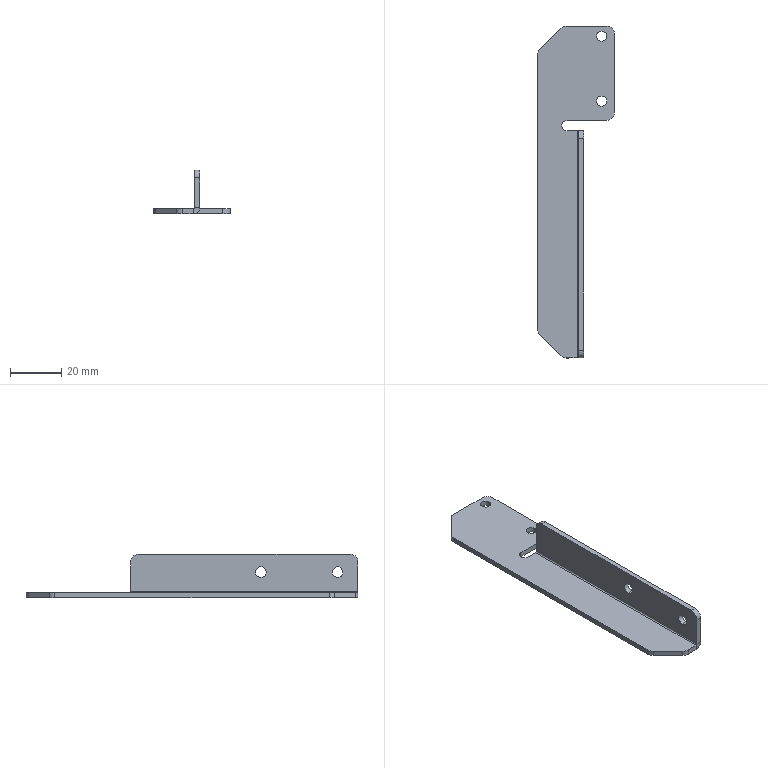Part | SolidWorks | features HoleWzd 2, EdgeFlange 1, Fillet 1, FlatPattern 1, SMBaseFlange 1, SheetMetal 1 | 1 solid | 36 faces | box 30 x 130 x 17 mm | volume 7736 mm3 | cylinder 19 | plane 17 | commonest cylinder face diameters 6 x8 4 x5 4.2 x4 1 x1 5 x1
STEP:
#1=CARTESIAN_POINT('',(23.,116.,-2.));
#2=VERTEX_POINT('',#1);
#3=CARTESIAN_POINT('',(27.,116.,-2.));
#4=VERTEX_POINT('',#3);
#5=CARTESIAN_POINT('',(25.,116.,-2.));
#6=DIRECTION('',(0.,0.,1.));
#7=DIRECTION('',(1.,0.,0.));
#8=AXIS2_PLACEMENT_3D('',#5,#6,#7);
#9=CIRCLE('',#8,2.);
#10=EDGE_CURVE('',#2,#4,#9,.T.);
#11=ORIENTED_EDGE('',*,*,#10,.F.);
#12=CARTESIAN_POINT('',(23.,116.,0.));
#13=VERTEX_POINT('',#12);
#14=CARTESIAN_POINT('',(23.,116.,0.));
#15=DIRECTION('',(0.,0.,1.));
#16=VECTOR('',#15,1000.);
#17=LINE('',#14,#16);
#18=EDGE_CURVE('',#2,#13,#17,.T.);
#19=ORIENTED_EDGE('',*,*,#18,.T.);
#20=CARTESIAN_POINT('',(27.,116.,0.));
#21=VERTEX_POINT('',#20);
#22=CARTESIAN_POINT('',(25.,116.,0.));
#23=DIRECTION('',(0.,0.,1.));
#24=DIRECTION('',(1.,0.,0.));
#25=AXIS2_PLACEMENT_3D('',#22,#23,#24);
#26=CIRCLE('',#25,2.);
#27=EDGE_CURVE('',#13,#21,#26,.T.);
#28=ORIENTED_EDGE('',*,*,#27,.T.);
#29=CARTESIAN_POINT('',(27.,116.,0.));
#30=DIRECTION('',(0.,0.,1.));
#31=VECTOR('',#30,1000.);
#32=LINE('',#29,#31);
#33=EDGE_CURVE('',#4,#21,#32,.T.);
#34=ORIENTED_EDGE('',*,*,#33,.F.);
#35=EDGE_LOOP('',(#11,#19,#28,#34));
#36=FACE_OUTER_BOUND('',#35,.T.);
#37=CARTESIAN_POINT('',(25.,116.,0.));
#38=DIRECTION('',(0.,0.,1.));
#39=DIRECTION('',(1.,0.,0.));
#40=AXIS2_PLACEMENT_3D('',#37,#38,#39);
#41=CYLINDRICAL_SURFACE('',#40,2.);
#42=ADVANCED_FACE('',(#36),#41,.F.);
#43=CARTESIAN_POINT('',(23.,90.6,-2.));
#44=VERTEX_POINT('',#43);
#45=CARTESIAN_POINT('',(27.,90.6,-2.));
#46=VERTEX_POINT('',#45);
#47=CARTESIAN_POINT('',(25.,90.6,-2.));
#48=DIRECTION('',(0.,0.,1.));
#49=DIRECTION('',(1.,0.,0.));
#50=AXIS2_PLACEMENT_3D('',#47,#48,#49);
#51=CIRCLE('',#50,2.);
#52=EDGE_CURVE('',#44,#46,#51,.T.);
#53=ORIENTED_EDGE('',*,*,#52,.F.);
#54=CARTESIAN_POINT('',(23.,90.6,0.));
#55=VERTEX_POINT('',#54);
#56=CARTESIAN_POINT('',(23.,90.6,0.));
#57=DIRECTION('',(0.,0.,1.));
#58=VECTOR('',#57,1000.);
#59=LINE('',#56,#58);
#60=EDGE_CURVE('',#44,#55,#59,.T.);
#61=ORIENTED_EDGE('',*,*,#60,.T.);
#62=CARTESIAN_POINT('',(27.,90.6,0.));
#63=VERTEX_POINT('',#62);
#64=CARTESIAN_POINT('',(25.,90.6,0.));
#65=DIRECTION('',(0.,0.,1.));
#66=DIRECTION('',(1.,0.,0.));
#67=AXIS2_PLACEMENT_3D('',#64,#65,#66);
#68=CIRCLE('',#67,2.);
#69=EDGE_CURVE('',#55,#63,#68,.T.);
#70=ORIENTED_EDGE('',*,*,#69,.T.);
#71=CARTESIAN_POINT('',(27.,90.6,0.));
#72=DIRECTION('',(0.,0.,1.));
#73=VECTOR('',#72,1000.);
#74=LINE('',#71,#73);
#75=EDGE_CURVE('',#46,#63,#74,.T.);
#76=ORIENTED_EDGE('',*,*,#75,.F.);
#77=EDGE_LOOP('',(#53,#61,#70,#76));
#78=FACE_OUTER_BOUND('',#77,.T.);
#79=CARTESIAN_POINT('',(25.,90.6,0.));
#80=DIRECTION('',(0.,0.,1.));
#81=DIRECTION('',(1.,0.,0.));
#82=AXIS2_PLACEMENT_3D('',#79,#80,#81);
#83=CYLINDRICAL_SURFACE('',#82,2.);
#84=ADVANCED_FACE('',(#78),#83,.F.);
#85=CARTESIAN_POINT('',(18.,28.,5.9));
#86=VERTEX_POINT('',#85);
#87=CARTESIAN_POINT('',(18.,28.,10.1));
#88=VERTEX_POINT('',#87);
#89=CARTESIAN_POINT('',(18.,28.,8.));
#90=DIRECTION('',(-1.,0.,0.));
#91=DIRECTION('',(0.,0.,1.));
#92=AXIS2_PLACEMENT_3D('',#89,#90,#91);
#93=CIRCLE('',#92,2.1);
#94=EDGE_CURVE('',#86,#88,#93,.T.);
#95=ORIENTED_EDGE('',*,*,#94,.F.);
#96=CARTESIAN_POINT('',(16.,28.,5.9));
#97=VERTEX_POINT('',#96);
#98=CARTESIAN_POINT('',(16.,28.,5.9));
#99=DIRECTION('',(-1.,0.,0.));
#100=VECTOR('',#99,1000.);
#101=LINE('',#98,#100);
#102=EDGE_CURVE('',#86,#97,#101,.T.);
#103=ORIENTED_EDGE('',*,*,#102,.T.);
#104=CARTESIAN_POINT('',(16.,28.,10.1));
#105=VERTEX_POINT('',#104);
#106=CARTESIAN_POINT('',(16.,28.,8.));
#107=DIRECTION('',(-1.,0.,0.));
#108=DIRECTION('',(0.,0.,1.));
#109=AXIS2_PLACEMENT_3D('',#106,#107,#108);
#110=CIRCLE('',#109,2.1);
#111=EDGE_CURVE('',#97,#105,#110,.T.);
#112=ORIENTED_EDGE('',*,*,#111,.T.);
#113=CARTESIAN_POINT('',(16.,28.,10.1));
#114=DIRECTION('',(-1.,0.,0.));
#115=VECTOR('',#114,1000.);
#116=LINE('',#113,#115);
#117=EDGE_CURVE('',#88,#105,#116,.T.);
#118=ORIENTED_EDGE('',*,*,#117,.F.);
#119=EDGE_LOOP('',(#95,#103,#112,#118));
#120=FACE_OUTER_BOUND('',#119,.T.);
#121=CARTESIAN_POINT('',(16.,28.,8.));
#122=DIRECTION('',(-1.,0.,0.));
#123=DIRECTION('',(0.,0.,1.));
#124=AXIS2_PLACEMENT_3D('',#121,#122,#123);
#125=CYLINDRICAL_SURFACE('',#124,2.1);
#126=ADVANCED_FACE('',(#120),#125,.F.);
#127=CARTESIAN_POINT('',(18.,-2.,5.9));
#128=VERTEX_POINT('',#127);
#129=CARTESIAN_POINT('',(18.,-2.,10.1));
#130=VERTEX_POINT('',#129);
#131=CARTESIAN_POINT('',(18.,-2.,8.));
#132=DIRECTION('',(-1.,0.,0.));
#133=DIRECTION('',(0.,0.,1.));
#134=AXIS2_PLACEMENT_3D('',#131,#132,#133);
#135=CIRCLE('',#134,2.1);
#136=EDGE_CURVE('',#128,#130,#135,.T.);
#137=ORIENTED_EDGE('',*,*,#136,.F.);
#138=CARTESIAN_POINT('',(16.,-2.,5.9));
#139=VERTEX_POINT('',#138);
#140=CARTESIAN_POINT('',(16.,-2.,5.9));
#141=DIRECTION('',(-1.,0.,0.));
#142=VECTOR('',#141,1000.);
#143=LINE('',#140,#142);
#144=EDGE_CURVE('',#128,#139,#143,.T.);
#145=ORIENTED_EDGE('',*,*,#144,.T.);
#146=CARTESIAN_POINT('',(16.,-2.,10.1));
#147=VERTEX_POINT('',#146);
#148=CARTESIAN_POINT('',(16.,-2.,8.));
#149=DIRECTION('',(-1.,0.,0.));
#150=DIRECTION('',(0.,0.,1.));
#151=AXIS2_PLACEMENT_3D('',#148,#149,#150);
#152=CIRCLE('',#151,2.1);
#153=EDGE_CURVE('',#139,#147,#152,.T.);
#154=ORIENTED_EDGE('',*,*,#153,.T.);
#155=CARTESIAN_POINT('',(16.,-2.,10.1));
#156=DIRECTION('',(-1.,0.,0.));
#157=VECTOR('',#156,1000.);
#158=LINE('',#155,#157);
#159=EDGE_CURVE('',#130,#147,#158,.T.);
#160=ORIENTED_EDGE('',*,*,#159,.F.);
#161=EDGE_LOOP('',(#137,#145,#154,#160));
#162=FACE_OUTER_BOUND('',#161,.T.);
#163=CARTESIAN_POINT('',(16.,-2.,8.));
#164=DIRECTION('',(-1.,0.,0.));
#165=DIRECTION('',(0.,0.,1.));
#166=AXIS2_PLACEMENT_3D('',#163,#164,#165);
#167=CYLINDRICAL_SURFACE('',#166,2.1);
#168=ADVANCED_FACE('',(#162),#167,.F.);
#169=CARTESIAN_POINT('',(30.,86.,0.));
#170=VERTEX_POINT('',#169);
#171=CARTESIAN_POINT('',(30.,117.,0.));
#172=VERTEX_POINT('',#171);
#173=CARTESIAN_POINT('',(30.,120.,0.));
#174=DIRECTION('',(0.,1.,0.));
#175=VECTOR('',#174,1000.);
#176=LINE('',#173,#175);
#177=EDGE_CURVE('',#170,#172,#176,.T.);
#178=ORIENTED_EDGE('',*,*,#177,.F.);
#179=CARTESIAN_POINT('',(30.,86.,-2.));
#180=VERTEX_POINT('',#179);
#181=CARTESIAN_POINT('',(30.,86.,-2.));
#182=DIRECTION('',(0.,0.,-1.));
#183=VECTOR('',#182,1000.);
#184=LINE('',#181,#183);
#185=EDGE_CURVE('',#170,#180,#184,.T.);
#186=ORIENTED_EDGE('',*,*,#185,.T.);
#187=CARTESIAN_POINT('',(30.,117.,-2.));
#188=VERTEX_POINT('',#187);
#189=CARTESIAN_POINT('',(30.,120.,-2.));
#190=DIRECTION('',(0.,1.,0.));
#191=VECTOR('',#190,1000.);
#192=LINE('',#189,#191);
#193=EDGE_CURVE('',#180,#188,#192,.T.);
#194=ORIENTED_EDGE('',*,*,#193,.T.);
#195=CARTESIAN_POINT('',(30.,117.,-2.));
#196=DIRECTION('',(0.,0.,1.));
#197=VECTOR('',#196,1000.);
#198=LINE('',#195,#197);
#199=EDGE_CURVE('',#188,#172,#198,.T.);
#200=ORIENTED_EDGE('',*,*,#199,.T.);
#201=EDGE_LOOP('',(#178,#186,#194,#200));
#202=FACE_OUTER_BOUND('',#201,.T.);
#203=CARTESIAN_POINT('',(30.,120.,-2.));
#204=DIRECTION('',(1.,0.,0.));
#205=DIRECTION('',(0.,1.,0.));
#206=AXIS2_PLACEMENT_3D('',#203,#204,#205);
#207=PLANE('',#206);
#208=ADVANCED_FACE('',(#202),#207,.T.);
#209=CARTESIAN_POINT('',(25.,116.,-2.));
#210=DIRECTION('',(0.,0.,1.));
#211=DIRECTION('',(1.,0.,0.));
#212=AXIS2_PLACEMENT_3D('',#209,#210,#211);
#213=CIRCLE('',#212,2.);
#214=EDGE_CURVE('',#4,#2,#213,.T.);
#215=ORIENTED_EDGE('',*,*,#214,.T.);
#216=ORIENTED_EDGE('',*,*,#10,.T.);
#217=EDGE_LOOP('',(#215,#216));
#218=FACE_BOUND('',#217,.T.);
#219=CARTESIAN_POINT('',(25.,90.6,-2.));
#220=DIRECTION('',(0.,0.,1.));
#221=DIRECTION('',(1.,0.,0.));
#222=AXIS2_PLACEMENT_3D('',#219,#220,#221);
#223=CIRCLE('',#222,2.);
#224=EDGE_CURVE('',#46,#44,#223,.T.);
#225=ORIENTED_EDGE('',*,*,#224,.T.);
#226=ORIENTED_EDGE('',*,*,#52,.T.);
#227=EDGE_LOOP('',(#225,#226));
#228=FACE_BOUND('',#227,.T.);
#229=CARTESIAN_POINT('',(0.8787,-0.8787,-2.));
#230=VERTEX_POINT('',#229);
#231=CARTESIAN_POINT('',(9.121,-9.121,-2.));
#232=VERTEX_POINT('',#231);
#233=CARTESIAN_POINT('',(0.,0.,-2.));
#234=DIRECTION('',(0.7071,-0.7071,0.));
#235=VECTOR('',#234,1000.);
#236=LINE('',#233,#235);
#237=EDGE_CURVE('',#230,#232,#236,.T.);
#238=ORIENTED_EDGE('',*,*,#237,.F.);
#239=CARTESIAN_POINT('',(0.,1.243,-2.));
#240=VERTEX_POINT('',#239);
#241=CARTESIAN_POINT('',(3.,1.243,-2.));
#242=DIRECTION('',(0.,0.,-1.));
#243=DIRECTION('',(1.,0.,0.));
#244=AXIS2_PLACEMENT_3D('',#241,#242,#243);
#245=CIRCLE('',#244,3.);
#246=EDGE_CURVE('',#230,#240,#245,.T.);
#247=ORIENTED_EDGE('',*,*,#246,.T.);
#248=CARTESIAN_POINT('',(0.,108.757,-2.));
#249=VERTEX_POINT('',#248);
#250=CARTESIAN_POINT('',(0.,0.,-2.));
#251=DIRECTION('',(0.,-1.,0.));
#252=VECTOR('',#251,1000.);
#253=LINE('',#250,#252);
#254=EDGE_CURVE('',#249,#240,#253,.T.);
#255=ORIENTED_EDGE('',*,*,#254,.F.);
#256=CARTESIAN_POINT('',(0.8787,110.879,-2.));
#257=VERTEX_POINT('',#256);
#258=CARTESIAN_POINT('',(3.,108.757,-2.));
#259=DIRECTION('',(0.,0.,-1.));
#260=DIRECTION('',(1.,0.,0.));
#261=AXIS2_PLACEMENT_3D('',#258,#259,#260);
#262=CIRCLE('',#261,3.);
#263=EDGE_CURVE('',#249,#257,#262,.T.);
#264=ORIENTED_EDGE('',*,*,#263,.T.);
#265=CARTESIAN_POINT('',(9.121,119.121,-2.));
#266=VERTEX_POINT('',#265);
#267=CARTESIAN_POINT('',(0.,110.,-2.));
#268=DIRECTION('',(-0.7071,-0.7071,0.));
#269=VECTOR('',#268,1000.);
#270=LINE('',#267,#269);
#271=EDGE_CURVE('',#266,#257,#270,.T.);
#272=ORIENTED_EDGE('',*,*,#271,.F.);
#273=CARTESIAN_POINT('',(11.243,120.,-2.));
#274=VERTEX_POINT('',#273);
#275=CARTESIAN_POINT('',(11.243,117.,-2.));
#276=DIRECTION('',(0.,0.,-1.));
#277=DIRECTION('',(1.,0.,0.));
#278=AXIS2_PLACEMENT_3D('',#275,#276,#277);
#279=CIRCLE('',#278,3.);
#280=EDGE_CURVE('',#266,#274,#279,.T.);
#281=ORIENTED_EDGE('',*,*,#280,.T.);
#282=CARTESIAN_POINT('',(27.,120.,-2.));
#283=VERTEX_POINT('',#282);
#284=CARTESIAN_POINT('',(10.,120.,-2.));
#285=DIRECTION('',(-1.,0.,0.));
#286=VECTOR('',#285,1000.);
#287=LINE('',#284,#286);
#288=EDGE_CURVE('',#283,#274,#287,.T.);
#289=ORIENTED_EDGE('',*,*,#288,.F.);
#290=CARTESIAN_POINT('',(27.,117.,-2.));
#291=DIRECTION('',(0.,0.,-1.));
#292=DIRECTION('',(1.,0.,0.));
#293=AXIS2_PLACEMENT_3D('',#290,#291,#292);
#294=CIRCLE('',#293,3.);
#295=EDGE_CURVE('',#283,#188,#294,.T.);
#296=ORIENTED_EDGE('',*,*,#295,.T.);
#297=ORIENTED_EDGE('',*,*,#193,.F.);
#298=CARTESIAN_POINT('',(27.,83.,-2.));
#299=VERTEX_POINT('',#298);
#300=CARTESIAN_POINT('',(27.,86.,-2.));
#301=DIRECTION('',(0.,0.,-1.));
#302=DIRECTION('',(1.,0.,0.));
#303=AXIS2_PLACEMENT_3D('',#300,#301,#302);
#304=CIRCLE('',#303,3.);
#305=EDGE_CURVE('',#180,#299,#304,.T.);
#306=ORIENTED_EDGE('',*,*,#305,.T.);
#307=CARTESIAN_POINT('',(11.5,83.,-2.));
#308=VERTEX_POINT('',#307);
#309=CARTESIAN_POINT('',(0.,83.,-2.));
#310=DIRECTION('',(1.,0.,0.));
#311=VECTOR('',#310,1000.);
#312=LINE('',#309,#311);
#313=EDGE_CURVE('',#308,#299,#312,.T.);
#314=ORIENTED_EDGE('',*,*,#313,.F.);
#315=CARTESIAN_POINT('',(11.5,79.,-2.));
#316=VERTEX_POINT('',#315);
#317=CARTESIAN_POINT('',(11.5,81.,-2.));
#318=DIRECTION('',(0.,0.,-1.));
#319=DIRECTION('',(1.,0.,0.));
#320=AXIS2_PLACEMENT_3D('',#317,#318,#319);
#321=CIRCLE('',#320,2.);
#322=EDGE_CURVE('',#316,#308,#321,.T.);
#323=ORIENTED_EDGE('',*,*,#322,.F.);
#324=CARTESIAN_POINT('',(15.5,79.,-2.));
#325=VERTEX_POINT('',#324);
#326=CARTESIAN_POINT('',(0.,79.,-2.));
#327=DIRECTION('',(-1.,0.,0.));
#328=VECTOR('',#327,1000.);
#329=LINE('',#326,#328);
#330=EDGE_CURVE('',#325,#316,#329,.T.);
#331=ORIENTED_EDGE('',*,*,#330,.F.);
#332=CARTESIAN_POINT('',(15.5,-10.,-2.));
#333=VERTEX_POINT('',#332);
#334=CARTESIAN_POINT('',(15.5,79.,-2.));
#335=DIRECTION('',(0.,-1.,0.));
#336=VECTOR('',#335,1000.);
#337=LINE('',#334,#336);
#338=EDGE_CURVE('',#325,#333,#337,.T.);
#339=ORIENTED_EDGE('',*,*,#338,.T.);
#340=CARTESIAN_POINT('',(11.243,-10.,-2.));
#341=VERTEX_POINT('',#340);
#342=CARTESIAN_POINT('',(10.,-10.,-2.));
#343=DIRECTION('',(1.,0.,0.));
#344=VECTOR('',#343,1000.);
#345=LINE('',#342,#344);
#346=EDGE_CURVE('',#341,#333,#345,.T.);
#347=ORIENTED_EDGE('',*,*,#346,.F.);
#348=CARTESIAN_POINT('',(11.243,-7.,-2.));
#349=DIRECTION('',(0.,0.,-1.));
#350=DIRECTION('',(1.,0.,0.));
#351=AXIS2_PLACEMENT_3D('',#348,#349,#350);
#352=CIRCLE('',#351,3.);
#353=EDGE_CURVE('',#341,#232,#352,.T.);
#354=ORIENTED_EDGE('',*,*,#353,.T.);
#355=EDGE_LOOP('',(#238,#247,#255,#264,#272,#281,#289,#296,#297,#306,#314,#323,#331,#339,#347,#354));
#356=FACE_OUTER_BOUND('',#355,.T.);
#357=CARTESIAN_POINT('',(0.,0.,-2.));
#358=DIRECTION('',(0.,0.,1.));
#359=DIRECTION('',(1.,0.,0.));
#360=AXIS2_PLACEMENT_3D('',#357,#358,#359);
#361=PLANE('',#360);
#362=ADVANCED_FACE('',(#218,#228,#356),#361,.F.);
#363=CARTESIAN_POINT('',(25.,116.,0.));
#364=DIRECTION('',(0.,0.,1.));
#365=DIRECTION('',(1.,0.,0.));
#366=AXIS2_PLACEMENT_3D('',#363,#364,#365);
#367=CIRCLE('',#366,2.);
#368=EDGE_CURVE('',#21,#13,#367,.T.);
#369=ORIENTED_EDGE('',*,*,#368,.F.);
#370=ORIENTED_EDGE('',*,*,#27,.F.);
#371=EDGE_LOOP('',(#369,#370));
#372=FACE_BOUND('',#371,.T.);
#373=CARTESIAN_POINT('',(25.,90.6,0.));
#374=DIRECTION('',(0.,0.,1.));
#375=DIRECTION('',(1.,0.,0.));
#376=AXIS2_PLACEMENT_3D('',#373,#374,#375);
#377=CIRCLE('',#376,2.);
#378=EDGE_CURVE('',#63,#55,#377,.T.);
#379=ORIENTED_EDGE('',*,*,#378,.F.);
#380=ORIENTED_EDGE('',*,*,#69,.F.);
#381=EDGE_LOOP('',(#379,#380));
#382=FACE_BOUND('',#381,.T.);
#383=CARTESIAN_POINT('',(0.,108.757,0.));
#384=VERTEX_POINT('',#383);
#385=CARTESIAN_POINT('',(0.,1.243,0.));
#386=VERTEX_POINT('',#385);
#387=CARTESIAN_POINT('',(0.,0.,0.));
#388=DIRECTION('',(0.,-1.,0.));
#389=VECTOR('',#388,1000.);
#390=LINE('',#387,#389);
#391=EDGE_CURVE('',#384,#386,#390,.T.);
#392=ORIENTED_EDGE('',*,*,#391,.T.);
#393=CARTESIAN_POINT('',(0.8787,-0.8787,0.));
#394=VERTEX_POINT('',#393);
#395=CARTESIAN_POINT('',(3.,1.243,0.));
#396=DIRECTION('',(0.,0.,1.));
#397=DIRECTION('',(1.,0.,0.));
#398=AXIS2_PLACEMENT_3D('',#395,#396,#397);
#399=CIRCLE('',#398,3.);
#400=EDGE_CURVE('',#386,#394,#399,.T.);
#401=ORIENTED_EDGE('',*,*,#400,.T.);
#402=CARTESIAN_POINT('',(9.121,-9.121,0.));
#403=VERTEX_POINT('',#402);
#404=CARTESIAN_POINT('',(0.,0.,0.));
#405=DIRECTION('',(0.7071,-0.7071,0.));
#406=VECTOR('',#405,1000.);
#407=LINE('',#404,#406);
#408=EDGE_CURVE('',#394,#403,#407,.T.);
#409=ORIENTED_EDGE('',*,*,#408,.T.);
#410=CARTESIAN_POINT('',(11.243,-10.,0.));
#411=VERTEX_POINT('',#410);
#412=CARTESIAN_POINT('',(11.243,-7.,0.));
#413=DIRECTION('',(0.,0.,1.));
#414=DIRECTION('',(1.,0.,0.));
#415=AXIS2_PLACEMENT_3D('',#412,#413,#414);
#416=CIRCLE('',#415,3.);
#417=EDGE_CURVE('',#403,#411,#416,.T.);
#418=ORIENTED_EDGE('',*,*,#417,.T.);
#419=CARTESIAN_POINT('',(15.5,-10.,0.));
#420=VERTEX_POINT('',#419);
#421=CARTESIAN_POINT('',(10.,-10.,0.));
#422=DIRECTION('',(1.,0.,0.));
#423=VECTOR('',#422,1000.);
#424=LINE('',#421,#423);
#425=EDGE_CURVE('',#411,#420,#424,.T.);
#426=ORIENTED_EDGE('',*,*,#425,.T.);
#427=CARTESIAN_POINT('',(15.5,79.,0.));
#428=VERTEX_POINT('',#427);
#429=CARTESIAN_POINT('',(15.5,79.,0.));
#430=DIRECTION('',(0.,-1.,0.));
#431=VECTOR('',#430,1000.);
#432=LINE('',#429,#431);
#433=EDGE_CURVE('',#428,#420,#432,.T.);
#434=ORIENTED_EDGE('',*,*,#433,.F.);
#435=CARTESIAN_POINT('',(11.5,79.,0.));
#436=VERTEX_POINT('',#435);
#437=CARTESIAN_POINT('',(11.5,79.,0.));
#438=DIRECTION('',(1.,0.,0.));
#439=VECTOR('',#438,1000.);
#440=LINE('',#437,#439);
#441=EDGE_CURVE('',#436,#428,#440,.T.);
#442=ORIENTED_EDGE('',*,*,#441,.F.);
#443=CARTESIAN_POINT('',(11.5,83.,0.));
#444=VERTEX_POINT('',#443);
#445=CARTESIAN_POINT('',(11.5,81.,0.));
#446=DIRECTION('',(0.,0.,1.));
#447=DIRECTION('',(1.,0.,0.));
#448=AXIS2_PLACEMENT_3D('',#445,#446,#447);
#449=CIRCLE('',#448,2.);
#450=EDGE_CURVE('',#444,#436,#449,.T.);
#451=ORIENTED_EDGE('',*,*,#450,.F.);
#452=CARTESIAN_POINT('',(27.,83.,0.));
#453=VERTEX_POINT('',#452);
#454=CARTESIAN_POINT('',(30.,83.,0.));
#455=DIRECTION('',(-1.,0.,0.));
#456=VECTOR('',#455,1000.);
#457=LINE('',#454,#456);
#458=EDGE_CURVE('',#453,#444,#457,.T.);
#459=ORIENTED_EDGE('',*,*,#458,.F.);
#460=CARTESIAN_POINT('',(27.,86.,0.));
#461=DIRECTION('',(0.,0.,1.));
#462=DIRECTION('',(1.,0.,0.));
#463=AXIS2_PLACEMENT_3D('',#460,#461,#462);
#464=CIRCLE('',#463,3.);
#465=EDGE_CURVE('',#453,#170,#464,.T.);
#466=ORIENTED_EDGE('',*,*,#465,.T.);
#467=ORIENTED_EDGE('',*,*,#177,.T.);
#468=CARTESIAN_POINT('',(27.,120.,0.));
#469=VERTEX_POINT('',#468);
#470=CARTESIAN_POINT('',(27.,117.,0.));
#471=DIRECTION('',(0.,0.,1.));
#472=DIRECTION('',(1.,0.,0.));
#473=AXIS2_PLACEMENT_3D('',#470,#471,#472);
#474=CIRCLE('',#473,3.);
#475=EDGE_CURVE('',#172,#469,#474,.T.);
#476=ORIENTED_EDGE('',*,*,#475,.T.);
#477=CARTESIAN_POINT('',(11.243,120.,0.));
#478=VERTEX_POINT('',#477);
#479=CARTESIAN_POINT('',(10.,120.,0.));
#480=DIRECTION('',(-1.,0.,0.));
#481=VECTOR('',#480,1000.);
#482=LINE('',#479,#481);
#483=EDGE_CURVE('',#469,#478,#482,.T.);
#484=ORIENTED_EDGE('',*,*,#483,.T.);
#485=CARTESIAN_POINT('',(9.121,119.121,0.));
#486=VERTEX_POINT('',#485);
#487=CARTESIAN_POINT('',(11.243,117.,0.));
#488=DIRECTION('',(0.,0.,1.));
#489=DIRECTION('',(1.,0.,0.));
#490=AXIS2_PLACEMENT_3D('',#487,#488,#489);
#491=CIRCLE('',#490,3.);
#492=EDGE_CURVE('',#478,#486,#491,.T.);
#493=ORIENTED_EDGE('',*,*,#492,.T.);
#494=CARTESIAN_POINT('',(0.8787,110.879,0.));
#495=VERTEX_POINT('',#494);
#496=CARTESIAN_POINT('',(0.,110.,0.));
#497=DIRECTION('',(-0.7071,-0.7071,0.));
#498=VECTOR('',#497,1000.);
#499=LINE('',#496,#498);
#500=EDGE_CURVE('',#486,#495,#499,.T.);
#501=ORIENTED_EDGE('',*,*,#500,.T.);
#502=CARTESIAN_POINT('',(3.,108.757,0.));
#503=DIRECTION('',(0.,0.,1.));
#504=DIRECTION('',(1.,0.,0.));
#505=AXIS2_PLACEMENT_3D('',#502,#503,#504);
#506=CIRCLE('',#505,3.);
#507=EDGE_CURVE('',#495,#384,#506,.T.);
#508=ORIENTED_EDGE('',*,*,#507,.T.);
#509=EDGE_LOOP('',(#392,#401,#409,#418,#426,#434,#442,#451,#459,#466,#467,#476,#484,#493,#501,#508));
#510=FACE_OUTER_BOUND('',#509,.T.);
#511=CARTESIAN_POINT('',(0.,0.,0.));
#512=DIRECTION('',(0.,0.,1.));
#513=DIRECTION('',(1.,0.,0.));
#514=AXIS2_PLACEMENT_3D('',#511,#512,#513);
#515=PLANE('',#514);
#516=ADVANCED_FACE('',(#372,#382,#510),#515,.T.);
#517=ORIENTED_EDGE('',*,*,#408,.F.);
#518=CARTESIAN_POINT('',(0.8787,-0.8787,-2.));
#519=DIRECTION('',(0.,0.,-1.));
#520=VECTOR('',#519,1000.);
#521=LINE('',#518,#520);
#522=EDGE_CURVE('',#394,#230,#521,.T.);
#523=ORIENTED_EDGE('',*,*,#522,.T.);
#524=ORIENTED_EDGE('',*,*,#237,.T.);
#525=CARTESIAN_POINT('',(9.121,-9.121,-2.));
#526=DIRECTION('',(0.,0.,1.));
#527=VECTOR('',#526,1000.);
#528=LINE('',#525,#527);
#529=EDGE_CURVE('',#232,#403,#528,.T.);
#530=ORIENTED_EDGE('',*,*,#529,.T.);
#531=EDGE_LOOP('',(#517,#523,#524,#530));
#532=FACE_OUTER_BOUND('',#531,.T.);
#533=CARTESIAN_POINT('',(0.,0.,-2.));
#534=DIRECTION('',(-0.7071,-0.7071,0.));
#535=DIRECTION('',(0.7071,-0.7071,0.));
#536=AXIS2_PLACEMENT_3D('',#533,#534,#535);
#537=PLANE('',#536);
#538=ADVANCED_FACE('',(#532),#537,.T.);
#539=ORIENTED_EDGE('',*,*,#254,.T.);
#540=CARTESIAN_POINT('',(0.,1.243,-2.));
#541=DIRECTION('',(0.,0.,1.));
#542=VECTOR('',#541,1000.);
#543=LINE('',#540,#542);
#544=EDGE_CURVE('',#240,#386,#543,.T.);
#545=ORIENTED_EDGE('',*,*,#544,.T.);
#546=ORIENTED_EDGE('',*,*,#391,.F.);
#547=CARTESIAN_POINT('',(0.,108.757,-2.));
#548=DIRECTION('',(0.,0.,-1.));
#549=VECTOR('',#548,1000.);
#550=LINE('',#547,#549);
#551=EDGE_CURVE('',#384,#249,#550,.T.);
#552=ORIENTED_EDGE('',*,*,#551,.T.);
#553=EDGE_LOOP('',(#539,#545,#546,#552));
#554=FACE_OUTER_BOUND('',#553,.T.);
#555=CARTESIAN_POINT('',(0.,0.,-2.));
#556=DIRECTION('',(-1.,0.,0.));
#557=DIRECTION('',(0.,0.,1.));
#558=AXIS2_PLACEMENT_3D('',#555,#556,#557);
#559=PLANE('',#558);
#560=ADVANCED_FACE('',(#554),#559,.T.);
#561=ORIENTED_EDGE('',*,*,#271,.T.);
#562=CARTESIAN_POINT('',(0.8787,110.879,-2.));
#563=DIRECTION('',(0.,0.,1.));
#564=VECTOR('',#563,1000.);
#565=LINE('',#562,#564);
#566=EDGE_CURVE('',#257,#495,#565,.T.);
#567=ORIENTED_EDGE('',*,*,#566,.T.);
#568=ORIENTED_EDGE('',*,*,#500,.F.);
#569=CARTESIAN_POINT('',(9.121,119.121,-2.));
#570=DIRECTION('',(0.,0.,-1.));
#571=VECTOR('',#570,1000.);
#572=LINE('',#569,#571);
#573=EDGE_CURVE('',#486,#266,#572,.T.);
#574=ORIENTED_EDGE('',*,*,#573,.T.);
#575=EDGE_LOOP('',(#561,#567,#568,#574));
#576=FACE_OUTER_BOUND('',#575,.T.);
#577=CARTESIAN_POINT('',(0.,110.,-2.));
#578=DIRECTION('',(-0.7071,0.7071,0.));
#579=DIRECTION('',(-0.7071,-0.7071,0.));
#580=AXIS2_PLACEMENT_3D('',#577,#578,#579);
#581=PLANE('',#580);
#582=ADVANCED_FACE('',(#576),#581,.T.);
#583=ORIENTED_EDGE('',*,*,#288,.T.);
#584=CARTESIAN_POINT('',(11.243,120.,-2.));
#585=DIRECTION('',(0.,0.,1.));
#586=VECTOR('',#585,1000.);
#587=LINE('',#584,#586);
#588=EDGE_CURVE('',#274,#478,#587,.T.);
#589=ORIENTED_EDGE('',*,*,#588,.T.);
#590=ORIENTED_EDGE('',*,*,#483,.F.);
#591=CARTESIAN_POINT('',(27.,120.,-2.));
#592=DIRECTION('',(0.,0.,-1.));
#593=VECTOR('',#592,1000.);
#594=LINE('',#591,#593);
#595=EDGE_CURVE('',#469,#283,#594,.T.);
#596=ORIENTED_EDGE('',*,*,#595,.T.);
#597=EDGE_LOOP('',(#583,#589,#590,#596));
#598=FACE_OUTER_BOUND('',#597,.T.);
#599=CARTESIAN_POINT('',(10.,120.,-2.));
#600=DIRECTION('',(0.,1.,0.));
#601=DIRECTION('',(0.,0.,1.));
#602=AXIS2_PLACEMENT_3D('',#599,#600,#601);
#603=PLANE('',#602);
#604=ADVANCED_FACE('',(#598),#603,.T.);
#605=ORIENTED_EDGE('',*,*,#425,.F.);
#606=CARTESIAN_POINT('',(11.243,-10.,-2.));
#607=DIRECTION('',(0.,0.,-1.));
#608=VECTOR('',#607,1000.);
#609=LINE('',#606,#608);
#610=EDGE_CURVE('',#411,#341,#609,.T.);
#611=ORIENTED_EDGE('',*,*,#610,.T.);
#612=ORIENTED_EDGE('',*,*,#346,.T.);
#613=CARTESIAN_POINT('',(15.5,-10.,0.));
#614=DIRECTION('',(0.,0.,-1.));
#615=VECTOR('',#614,1000.);
#616=LINE('',#613,#615);
#617=EDGE_CURVE('',#420,#333,#616,.T.);
#618=ORIENTED_EDGE('',*,*,#617,.F.);
#619=EDGE_LOOP('',(#605,#611,#612,#618));
#620=FACE_OUTER_BOUND('',#619,.T.);
#621=CARTESIAN_POINT('',(10.,-10.,-2.));
#622=DIRECTION('',(0.,-1.,0.));
#623=DIRECTION('',(1.,0.,0.));
#624=AXIS2_PLACEMENT_3D('',#621,#622,#623);
#625=PLANE('',#624);
#626=ADVANCED_FACE('',(#620),#625,.T.);
#627=ORIENTED_EDGE('',*,*,#313,.T.);
#628=CARTESIAN_POINT('',(27.,83.,0.));
#629=DIRECTION('',(0.,0.,1.));
#630=VECTOR('',#629,1000.);
#631=LINE('',#628,#630);
#632=EDGE_CURVE('',#299,#453,#631,.T.);
#633=ORIENTED_EDGE('',*,*,#632,.T.);
#634=ORIENTED_EDGE('',*,*,#458,.T.);
#635=CARTESIAN_POINT('',(11.5,83.,0.));
#636=DIRECTION('',(0.,0.,-1.));
#637=VECTOR('',#636,1000.);
#638=LINE('',#635,#637);
#639=EDGE_CURVE('',#444,#308,#638,.T.);
#640=ORIENTED_EDGE('',*,*,#639,.T.);
#641=EDGE_LOOP('',(#627,#633,#634,#640));
#642=FACE_OUTER_BOUND('',#641,.T.);
#643=CARTESIAN_POINT('',(30.,83.,0.));
#644=DIRECTION('',(0.,-1.,0.));
#645=DIRECTION('',(0.,0.,-1.));
#646=AXIS2_PLACEMENT_3D('',#643,#644,#645);
#647=PLANE('',#646);
#648=ADVANCED_FACE('',(#642),#647,.T.);
#649=CARTESIAN_POINT('',(11.5,79.,0.));
#650=DIRECTION('',(0.,0.,-1.));
#651=VECTOR('',#650,1000.);
#652=LINE('',#649,#651);
#653=EDGE_CURVE('',#436,#316,#652,.T.);
#654=ORIENTED_EDGE('',*,*,#653,.T.);
#655=ORIENTED_EDGE('',*,*,#322,.T.);
#656=ORIENTED_EDGE('',*,*,#639,.F.);
#657=ORIENTED_EDGE('',*,*,#450,.T.);
#658=EDGE_LOOP('',(#654,#655,#656,#657));
#659=FACE_OUTER_BOUND('',#658,.T.);
#660=CARTESIAN_POINT('',(11.5,81.,0.));
#661=DIRECTION('',(0.,0.,-1.));
#662=DIRECTION('',(0.,1.,0.));
#663=AXIS2_PLACEMENT_3D('',#660,#661,#662);
#664=CYLINDRICAL_SURFACE('',#663,2.);
#665=ADVANCED_FACE('',(#659),#664,.F.);
#666=CARTESIAN_POINT('',(15.5,79.,0.));
#667=DIRECTION('',(0.,0.,-1.));
#668=VECTOR('',#667,1000.);
#669=LINE('',#666,#668);
#670=EDGE_CURVE('',#428,#325,#669,.T.);
#671=ORIENTED_EDGE('',*,*,#670,.T.);
#672=ORIENTED_EDGE('',*,*,#330,.T.);
#673=ORIENTED_EDGE('',*,*,#653,.F.);
#674=ORIENTED_EDGE('',*,*,#441,.T.);
#675=EDGE_LOOP('',(#671,#672,#673,#674));
#676=FACE_OUTER_BOUND('',#675,.T.);
#677=CARTESIAN_POINT('',(11.5,79.,0.));
#678=DIRECTION('',(0.,1.,0.));
#679=DIRECTION('',(0.,0.,1.));
#680=AXIS2_PLACEMENT_3D('',#677,#678,#679);
#681=PLANE('',#680);
#682=ADVANCED_FACE('',(#676),#681,.T.);
#683=CARTESIAN_POINT('',(16.,-10.,0.5));
#684=VERTEX_POINT('',#683);
#685=CARTESIAN_POINT('',(18.,-10.,0.5));
#686=VERTEX_POINT('',#685);
#687=CARTESIAN_POINT('',(18.,-10.,0.5));
#688=DIRECTION('',(1.,0.,0.));
#689=VECTOR('',#688,1000.);
#690=LINE('',#687,#689);
#691=EDGE_CURVE('',#684,#686,#690,.T.);
#692=ORIENTED_EDGE('',*,*,#691,.F.);
#693=CARTESIAN_POINT('',(15.5,-10.,0.5));
#694=DIRECTION('',(0.,-1.,0.));
#695=DIRECTION('',(0.,0.,1.));
#696=AXIS2_PLACEMENT_3D('',#693,#694,#695);
#697=CIRCLE('',#696,0.5);
#698=EDGE_CURVE('',#420,#684,#697,.T.);
#699=ORIENTED_EDGE('',*,*,#698,.F.);
#700=ORIENTED_EDGE('',*,*,#617,.T.);
#701=CARTESIAN_POINT('',(15.5,-10.,0.5));
#702=DIRECTION('',(0.,-1.,0.));
#703=DIRECTION('',(0.,0.,1.));
#704=AXIS2_PLACEMENT_3D('',#701,#702,#703);
#705=CIRCLE('',#704,2.5);
#706=EDGE_CURVE('',#333,#686,#705,.T.);
#707=ORIENTED_EDGE('',*,*,#706,.T.);
#708=EDGE_LOOP('',(#692,#699,#700,#707));
#709=FACE_OUTER_BOUND('',#708,.T.);
#710=CARTESIAN_POINT('',(15.5,-10.,0.5));
#711=DIRECTION('',(0.,-1.,0.));
#712=DIRECTION('',(0.,0.,-1.));
#713=AXIS2_PLACEMENT_3D('',#710,#711,#712);
#714=PLANE('',#713);
#715=ADVANCED_FACE('',(#709),#714,.T.);
#716=CARTESIAN_POINT('',(16.,79.,0.5));
#717=VERTEX_POINT('',#716);
#718=CARTESIAN_POINT('',(15.5,79.,0.5));
#719=DIRECTION('',(0.,1.,0.));
#720=DIRECTION('',(0.,0.,1.));
#721=AXIS2_PLACEMENT_3D('',#718,#719,#720);
#722=CIRCLE('',#721,0.5);
#723=EDGE_CURVE('',#717,#428,#722,.T.);
#724=ORIENTED_EDGE('',*,*,#723,.F.);
#725=CARTESIAN_POINT('',(18.,79.,0.5));
#726=VERTEX_POINT('',#725);
#727=CARTESIAN_POINT('',(16.,79.,0.5));
#728=DIRECTION('',(1.,0.,0.));
#729=VECTOR('',#728,1000.);
#730=LINE('',#727,#729);
#731=EDGE_CURVE('',#717,#726,#730,.T.);
#732=ORIENTED_EDGE('',*,*,#731,.T.);
#733=CARTESIAN_POINT('',(15.5,79.,0.5));
#734=DIRECTION('',(0.,1.,0.));
#735=DIRECTION('',(0.,0.,1.));
#736=AXIS2_PLACEMENT_3D('',#733,#734,#735);
#737=CIRCLE('',#736,2.5);
#738=EDGE_CURVE('',#726,#325,#737,.T.);
#739=ORIENTED_EDGE('',*,*,#738,.T.);
#740=ORIENTED_EDGE('',*,*,#670,.F.);
#741=EDGE_LOOP('',(#724,#732,#739,#740));
#742=FACE_OUTER_BOUND('',#741,.T.);
#743=CARTESIAN_POINT('',(15.5,79.,0.5));
#744=DIRECTION('',(0.,-1.,0.));
#745=DIRECTION('',(0.,0.,-1.));
#746=AXIS2_PLACEMENT_3D('',#743,#744,#745);
#747=PLANE('',#746);
#748=ADVANCED_FACE('',(#742),#747,.F.);
#749=ORIENTED_EDGE('',*,*,#338,.F.);
#750=ORIENTED_EDGE('',*,*,#738,.F.);
#751=CARTESIAN_POINT('',(18.,-10.,0.5));
#752=DIRECTION('',(0.,-1.,0.));
#753=VECTOR('',#752,1000.);
#754=LINE('',#751,#753);
#755=EDGE_CURVE('',#726,#686,#754,.T.);
#756=ORIENTED_EDGE('',*,*,#755,.T.);
#757=ORIENTED_EDGE('',*,*,#706,.F.);
#758=EDGE_LOOP('',(#749,#750,#756,#757));
#759=FACE_OUTER_BOUND('',#758,.T.);
#760=CARTESIAN_POINT('',(15.5,79.,0.5));
#761=DIRECTION('',(0.,1.,0.));
#762=DIRECTION('',(1.,0.,0.));
#763=AXIS2_PLACEMENT_3D('',#760,#761,#762);
#764=CYLINDRICAL_SURFACE('',#763,2.5);
#765=ADVANCED_FACE('',(#759),#764,.T.);
#766=ORIENTED_EDGE('',*,*,#433,.T.);
#767=ORIENTED_EDGE('',*,*,#698,.T.);
#768=CARTESIAN_POINT('',(16.,-10.,0.5));
#769=DIRECTION('',(0.,1.,0.));
#770=VECTOR('',#769,1000.);
#771=LINE('',#768,#770);
#772=EDGE_CURVE('',#684,#717,#771,.T.);
#773=ORIENTED_EDGE('',*,*,#772,.T.);
#774=ORIENTED_EDGE('',*,*,#723,.T.);
#775=EDGE_LOOP('',(#766,#767,#773,#774));
#776=FACE_OUTER_BOUND('',#775,.T.);
#777=CARTESIAN_POINT('',(15.5,79.,0.5));
#778=DIRECTION('',(0.,1.,0.));
#779=DIRECTION('',(1.,0.,0.));
#780=AXIS2_PLACEMENT_3D('',#777,#778,#779);
#781=CYLINDRICAL_SURFACE('',#780,0.5);
#782=ADVANCED_FACE('',(#776),#781,.F.);
#783=CARTESIAN_POINT('',(16.,79.,12.));
#784=VERTEX_POINT('',#783);
#785=CARTESIAN_POINT('',(16.,79.,15.));
#786=DIRECTION('',(0.,0.,1.));
#787=VECTOR('',#786,1000.);
#788=LINE('',#785,#787);
#789=EDGE_CURVE('',#717,#784,#788,.T.);
#790=ORIENTED_EDGE('',*,*,#789,.T.);
#791=CARTESIAN_POINT('',(18.,79.,12.));
#792=VERTEX_POINT('',#791);
#793=CARTESIAN_POINT('',(18.,79.,12.));
#794=DIRECTION('',(1.,0.,0.));
#795=VECTOR('',#794,1000.);
#796=LINE('',#793,#795);
#797=EDGE_CURVE('',#784,#792,#796,.T.);
#798=ORIENTED_EDGE('',*,*,#797,.T.);
#799=CARTESIAN_POINT('',(18.,79.,0.));
#800=DIRECTION('',(0.,0.,1.));
#801=VECTOR('',#800,1000.);
#802=LINE('',#799,#801);
#803=EDGE_CURVE('',#726,#792,#802,.T.);
#804=ORIENTED_EDGE('',*,*,#803,.F.);
#805=ORIENTED_EDGE('',*,*,#731,.F.);
#806=EDGE_LOOP('',(#790,#798,#804,#805));
#807=FACE_OUTER_BOUND('',#806,.T.);
#808=CARTESIAN_POINT('',(18.,79.,15.));
#809=DIRECTION('',(0.,-1.,0.));
#810=DIRECTION('',(1.,0.,0.));
#811=AXIS2_PLACEMENT_3D('',#808,#809,#810);
#812=PLANE('',#811);
#813=ADVANCED_FACE('',(#807),#812,.F.);
#814=CARTESIAN_POINT('',(18.,-10.,12.));
#815=VERTEX_POINT('',#814);
#816=CARTESIAN_POINT('',(18.,-10.,0.));
#817=DIRECTION('',(0.,0.,-1.));
#818=VECTOR('',#817,1000.);
#819=LINE('',#816,#818);
#820=EDGE_CURVE('',#815,#686,#819,.T.);
#821=ORIENTED_EDGE('',*,*,#820,.F.);
#822=CARTESIAN_POINT('',(16.,-10.,12.));
#823=VERTEX_POINT('',#822);
#824=CARTESIAN_POINT('',(18.,-10.,12.));
#825=DIRECTION('',(-1.,0.,0.));
#826=VECTOR('',#825,1000.);
#827=LINE('',#824,#826);
#828=EDGE_CURVE('',#815,#823,#827,.T.);
#829=ORIENTED_EDGE('',*,*,#828,.T.);
#830=CARTESIAN_POINT('',(16.,-10.,0.));
#831=DIRECTION('',(0.,0.,-1.));
#832=VECTOR('',#831,1000.);
#833=LINE('',#830,#832);
#834=EDGE_CURVE('',#823,#684,#833,.T.);
#835=ORIENTED_EDGE('',*,*,#834,.T.);
#836=ORIENTED_EDGE('',*,*,#691,.T.);
#837=EDGE_LOOP('',(#821,#829,#835,#836));
#838=FACE_OUTER_BOUND('',#837,.T.);
#839=CARTESIAN_POINT('',(18.,-10.,0.));
#840=DIRECTION('',(0.,1.,0.));
#841=DIRECTION('',(0.,0.,1.));
#842=AXIS2_PLACEMENT_3D('',#839,#840,#841);
#843=PLANE('',#842);
#844=ADVANCED_FACE('',(#838),#843,.F.);
#845=CARTESIAN_POINT('',(18.,28.,8.));
#846=DIRECTION('',(-1.,0.,0.));
#847=DIRECTION('',(0.,0.,1.));
#848=AXIS2_PLACEMENT_3D('',#845,#846,#847);
#849=CIRCLE('',#848,2.1);
#850=EDGE_CURVE('',#88,#86,#849,.T.);
#851=ORIENTED_EDGE('',*,*,#850,.T.);
#852=ORIENTED_EDGE('',*,*,#94,.T.);
#853=EDGE_LOOP('',(#851,#852));
#854=FACE_BOUND('',#853,.T.);
#855=CARTESIAN_POINT('',(18.,-2.,8.));
#856=DIRECTION('',(-1.,0.,0.));
#857=DIRECTION('',(0.,0.,1.));
#858=AXIS2_PLACEMENT_3D('',#855,#856,#857);
#859=CIRCLE('',#858,2.1);
#860=EDGE_CURVE('',#130,#128,#859,.T.);
#861=ORIENTED_EDGE('',*,*,#860,.T.);
#862=ORIENTED_EDGE('',*,*,#136,.T.);
#863=EDGE_LOOP('',(#861,#862));
#864=FACE_BOUND('',#863,.T.);
#865=CARTESIAN_POINT('',(18.,76.,15.));
#866=VERTEX_POINT('',#865);
#867=CARTESIAN_POINT('',(18.,-7.,15.));
#868=VERTEX_POINT('',#867);
#869=CARTESIAN_POINT('',(18.,0.,15.));
#870=DIRECTION('',(0.,-1.,0.));
#871=VECTOR('',#870,1000.);
#872=LINE('',#869,#871);
#873=EDGE_CURVE('',#866,#868,#872,.T.);
#874=ORIENTED_EDGE('',*,*,#873,.T.);
#875=CARTESIAN_POINT('',(18.,-7.,12.));
#876=DIRECTION('',(1.,0.,0.));
#877=DIRECTION('',(0.,0.,1.));
#878=AXIS2_PLACEMENT_3D('',#875,#876,#877);
#879=CIRCLE('',#878,3.);
#880=EDGE_CURVE('',#868,#815,#879,.T.);
#881=ORIENTED_EDGE('',*,*,#880,.T.);
#882=ORIENTED_EDGE('',*,*,#820,.T.);
#883=ORIENTED_EDGE('',*,*,#755,.F.);
#884=ORIENTED_EDGE('',*,*,#803,.T.);
#885=CARTESIAN_POINT('',(18.,76.,12.));
#886=DIRECTION('',(1.,0.,0.));
#887=DIRECTION('',(0.,0.,1.));
#888=AXIS2_PLACEMENT_3D('',#885,#886,#887);
#889=CIRCLE('',#888,3.);
#890=EDGE_CURVE('',#792,#866,#889,.T.);
#891=ORIENTED_EDGE('',*,*,#890,.T.);
#892=EDGE_LOOP('',(#874,#881,#882,#883,#884,#891));
#893=FACE_OUTER_BOUND('',#892,.T.);
#894=CARTESIAN_POINT('',(18.,0.,0.));
#895=DIRECTION('',(-1.,0.,0.));
#896=DIRECTION('',(0.,0.,1.));
#897=AXIS2_PLACEMENT_3D('',#894,#895,#896);
#898=PLANE('',#897);
#899=ADVANCED_FACE('',(#854,#864,#893),#898,.F.);
#900=CARTESIAN_POINT('',(16.,28.,8.));
#901=DIRECTION('',(-1.,0.,0.));
#902=DIRECTION('',(0.,0.,1.));
#903=AXIS2_PLACEMENT_3D('',#900,#901,#902);
#904=CIRCLE('',#903,2.1);
#905=EDGE_CURVE('',#105,#97,#904,.T.);
#906=ORIENTED_EDGE('',*,*,#905,.F.);
#907=ORIENTED_EDGE('',*,*,#111,.F.);
#908=EDGE_LOOP('',(#906,#907));
#909=FACE_BOUND('',#908,.T.);
#910=CARTESIAN_POINT('',(16.,-2.,8.));
#911=DIRECTION('',(-1.,0.,0.));
#912=DIRECTION('',(0.,0.,1.));
#913=AXIS2_PLACEMENT_3D('',#910,#911,#912);
#914=CIRCLE('',#913,2.1);
#915=EDGE_CURVE('',#147,#139,#914,.T.);
#916=ORIENTED_EDGE('',*,*,#915,.F.);
#917=ORIENTED_EDGE('',*,*,#153,.F.);
#918=EDGE_LOOP('',(#916,#917));
#919=FACE_BOUND('',#918,.T.);
#920=ORIENTED_EDGE('',*,*,#834,.F.);
#921=CARTESIAN_POINT('',(16.,-7.,15.));
#922=VERTEX_POINT('',#921);
#923=CARTESIAN_POINT('',(16.,-7.,12.));
#924=DIRECTION('',(-1.,0.,0.));
#925=DIRECTION('',(0.,0.,1.));
#926=AXIS2_PLACEMENT_3D('',#923,#924,#925);
#927=CIRCLE('',#926,3.);
#928=EDGE_CURVE('',#823,#922,#927,.T.);
#929=ORIENTED_EDGE('',*,*,#928,.T.);
#930=CARTESIAN_POINT('',(16.,76.,15.));
#931=VERTEX_POINT('',#930);
#932=CARTESIAN_POINT('',(16.,-10.,15.));
#933=DIRECTION('',(0.,-1.,0.));
#934=VECTOR('',#933,1000.);
#935=LINE('',#932,#934);
#936=EDGE_CURVE('',#931,#922,#935,.T.);
#937=ORIENTED_EDGE('',*,*,#936,.F.);
#938=CARTESIAN_POINT('',(16.,76.,12.));
#939=DIRECTION('',(-1.,0.,0.));
#940=DIRECTION('',(0.,0.,1.));
#941=AXIS2_PLACEMENT_3D('',#938,#939,#940);
#942=CIRCLE('',#941,3.);
#943=EDGE_CURVE('',#931,#784,#942,.T.);
#944=ORIENTED_EDGE('',*,*,#943,.T.);
#945=ORIENTED_EDGE('',*,*,#789,.F.);
#946=ORIENTED_EDGE('',*,*,#772,.F.);
#947=EDGE_LOOP('',(#920,#929,#937,#944,#945,#946));
#948=FACE_OUTER_BOUND('',#947,.T.);
#949=CARTESIAN_POINT('',(16.,0.,0.));
#950=DIRECTION('',(-1.,0.,0.));
#951=DIRECTION('',(0.,0.,1.));
#952=AXIS2_PLACEMENT_3D('',#949,#950,#951);
#953=PLANE('',#952);
#954=ADVANCED_FACE('',(#909,#919,#948),#953,.T.);
#955=ORIENTED_EDGE('',*,*,#936,.T.);
#956=CARTESIAN_POINT('',(18.,-7.,15.));
#957=DIRECTION('',(1.,0.,0.));
#958=VECTOR('',#957,1000.);
#959=LINE('',#956,#958);
#960=EDGE_CURVE('',#922,#868,#959,.T.);
#961=ORIENTED_EDGE('',*,*,#960,.T.);
#962=ORIENTED_EDGE('',*,*,#873,.F.);
#963=CARTESIAN_POINT('',(18.,76.,15.));
#964=DIRECTION('',(-1.,0.,0.));
#965=VECTOR('',#964,1000.);
#966=LINE('',#963,#965);
#967=EDGE_CURVE('',#866,#931,#966,.T.);
#968=ORIENTED_EDGE('',*,*,#967,.T.);
#969=EDGE_LOOP('',(#955,#961,#962,#968));
#970=FACE_OUTER_BOUND('',#969,.T.);
#971=CARTESIAN_POINT('',(18.,-10.,15.));
#972=DIRECTION('',(0.,0.,-1.));
#973=DIRECTION('',(-1.,0.,0.));
#974=AXIS2_PLACEMENT_3D('',#971,#972,#973);
#975=PLANE('',#974);
#976=ADVANCED_FACE('',(#970),#975,.F.);
#977=ORIENTED_EDGE('',*,*,#144,.F.);
#978=ORIENTED_EDGE('',*,*,#860,.F.);
#979=ORIENTED_EDGE('',*,*,#159,.T.);
#980=ORIENTED_EDGE('',*,*,#915,.T.);
#981=EDGE_LOOP('',(#977,#978,#979,#980));
#982=FACE_OUTER_BOUND('',#981,.T.);
#983=CARTESIAN_POINT('',(16.,-2.,8.));
#984=DIRECTION('',(-1.,0.,0.));
#985=DIRECTION('',(0.,0.,1.));
#986=AXIS2_PLACEMENT_3D('',#983,#984,#985);
#987=CYLINDRICAL_SURFACE('',#986,2.1);
#988=ADVANCED_FACE('',(#982),#987,.F.);
#989=ORIENTED_EDGE('',*,*,#102,.F.);
#990=ORIENTED_EDGE('',*,*,#850,.F.);
#991=ORIENTED_EDGE('',*,*,#117,.T.);
#992=ORIENTED_EDGE('',*,*,#905,.T.);
#993=EDGE_LOOP('',(#989,#990,#991,#992));
#994=FACE_OUTER_BOUND('',#993,.T.);
#995=CARTESIAN_POINT('',(16.,28.,8.));
#996=DIRECTION('',(-1.,0.,0.));
#997=DIRECTION('',(0.,0.,1.));
#998=AXIS2_PLACEMENT_3D('',#995,#996,#997);
#999=CYLINDRICAL_SURFACE('',#998,2.1);
#1000=ADVANCED_FACE('',(#994),#999,.F.);
#1001=ORIENTED_EDGE('',*,*,#60,.F.);
#1002=ORIENTED_EDGE('',*,*,#224,.F.);
#1003=ORIENTED_EDGE('',*,*,#75,.T.);
#1004=ORIENTED_EDGE('',*,*,#378,.T.);
#1005=EDGE_LOOP('',(#1001,#1002,#1003,#1004));
#1006=FACE_OUTER_BOUND('',#1005,.T.);
#1007=CARTESIAN_POINT('',(25.,90.6,0.));
#1008=DIRECTION('',(0.,0.,1.));
#1009=DIRECTION('',(1.,0.,0.));
#1010=AXIS2_PLACEMENT_3D('',#1007,#1008,#1009);
#1011=CYLINDRICAL_SURFACE('',#1010,2.);
#1012=ADVANCED_FACE('',(#1006),#1011,.F.);
#1013=ORIENTED_EDGE('',*,*,#18,.F.);
#1014=ORIENTED_EDGE('',*,*,#214,.F.);
#1015=ORIENTED_EDGE('',*,*,#33,.T.);
#1016=ORIENTED_EDGE('',*,*,#368,.T.);
#1017=EDGE_LOOP('',(#1013,#1014,#1015,#1016));
#1018=FACE_OUTER_BOUND('',#1017,.T.);
#1019=CARTESIAN_POINT('',(25.,116.,0.));
#1020=DIRECTION('',(0.,0.,1.));
#1021=DIRECTION('',(1.,0.,0.));
#1022=AXIS2_PLACEMENT_3D('',#1019,#1020,#1021);
#1023=CYLINDRICAL_SURFACE('',#1022,2.);
#1024=ADVANCED_FACE('',(#1018),#1023,.F.);
#1025=ORIENTED_EDGE('',*,*,#246,.F.);
#1026=ORIENTED_EDGE('',*,*,#522,.F.);
#1027=ORIENTED_EDGE('',*,*,#400,.F.);
#1028=ORIENTED_EDGE('',*,*,#544,.F.);
#1029=EDGE_LOOP('',(#1025,#1026,#1027,#1028));
#1030=FACE_OUTER_BOUND('',#1029,.T.);
#1031=CARTESIAN_POINT('',(3.,1.243,-2.));
#1032=DIRECTION('',(0.,0.,1.));
#1033=DIRECTION('',(1.,0.,0.));
#1034=AXIS2_PLACEMENT_3D('',#1031,#1032,#1033);
#1035=CYLINDRICAL_SURFACE('',#1034,3.);
#1036=ADVANCED_FACE('',(#1030),#1035,.T.);
#1037=ORIENTED_EDGE('',*,*,#353,.F.);
#1038=ORIENTED_EDGE('',*,*,#610,.F.);
#1039=ORIENTED_EDGE('',*,*,#417,.F.);
#1040=ORIENTED_EDGE('',*,*,#529,.F.);
#1041=EDGE_LOOP('',(#1037,#1038,#1039,#1040));
#1042=FACE_OUTER_BOUND('',#1041,.T.);
#1043=CARTESIAN_POINT('',(11.243,-7.,-2.));
#1044=DIRECTION('',(0.,0.,1.));
#1045=DIRECTION('',(1.,0.,0.));
#1046=AXIS2_PLACEMENT_3D('',#1043,#1044,#1045);
#1047=CYLINDRICAL_SURFACE('',#1046,3.);
#1048=ADVANCED_FACE('',(#1042),#1047,.T.);
#1049=ORIENTED_EDGE('',*,*,#880,.F.);
#1050=ORIENTED_EDGE('',*,*,#960,.F.);
#1051=ORIENTED_EDGE('',*,*,#928,.F.);
#1052=ORIENTED_EDGE('',*,*,#828,.F.);
#1053=EDGE_LOOP('',(#1049,#1050,#1051,#1052));
#1054=FACE_OUTER_BOUND('',#1053,.T.);
#1055=CARTESIAN_POINT('',(18.,-7.,12.));
#1056=DIRECTION('',(-1.,0.,0.));
#1057=DIRECTION('',(0.,0.,1.));
#1058=AXIS2_PLACEMENT_3D('',#1055,#1056,#1057);
#1059=CYLINDRICAL_SURFACE('',#1058,3.);
#1060=ADVANCED_FACE('',(#1054),#1059,.T.);
#1061=ORIENTED_EDGE('',*,*,#890,.F.);
#1062=ORIENTED_EDGE('',*,*,#797,.F.);
#1063=ORIENTED_EDGE('',*,*,#943,.F.);
#1064=ORIENTED_EDGE('',*,*,#967,.F.);
#1065=EDGE_LOOP('',(#1061,#1062,#1063,#1064));
#1066=FACE_OUTER_BOUND('',#1065,.T.);
#1067=CARTESIAN_POINT('',(18.,76.,12.));
#1068=DIRECTION('',(-1.,0.,0.));
#1069=DIRECTION('',(0.,0.,1.));
#1070=AXIS2_PLACEMENT_3D('',#1067,#1068,#1069);
#1071=CYLINDRICAL_SURFACE('',#1070,3.);
#1072=ADVANCED_FACE('',(#1066),#1071,.T.);
#1073=ORIENTED_EDGE('',*,*,#263,.F.);
#1074=ORIENTED_EDGE('',*,*,#551,.F.);
#1075=ORIENTED_EDGE('',*,*,#507,.F.);
#1076=ORIENTED_EDGE('',*,*,#566,.F.);
#1077=EDGE_LOOP('',(#1073,#1074,#1075,#1076));
#1078=FACE_OUTER_BOUND('',#1077,.T.);
#1079=CARTESIAN_POINT('',(3.,108.757,-2.));
#1080=DIRECTION('',(0.,0.,1.));
#1081=DIRECTION('',(1.,0.,0.));
#1082=AXIS2_PLACEMENT_3D('',#1079,#1080,#1081);
#1083=CYLINDRICAL_SURFACE('',#1082,3.);
#1084=ADVANCED_FACE('',(#1078),#1083,.T.);
#1085=ORIENTED_EDGE('',*,*,#280,.F.);
#1086=ORIENTED_EDGE('',*,*,#573,.F.);
#1087=ORIENTED_EDGE('',*,*,#492,.F.);
#1088=ORIENTED_EDGE('',*,*,#588,.F.);
#1089=EDGE_LOOP('',(#1085,#1086,#1087,#1088));
#1090=FACE_OUTER_BOUND('',#1089,.T.);
#1091=CARTESIAN_POINT('',(11.243,117.,-2.));
#1092=DIRECTION('',(0.,0.,1.));
#1093=DIRECTION('',(1.,0.,0.));
#1094=AXIS2_PLACEMENT_3D('',#1091,#1092,#1093);
#1095=CYLINDRICAL_SURFACE('',#1094,3.);
#1096=ADVANCED_FACE('',(#1090),#1095,.T.);
#1097=ORIENTED_EDGE('',*,*,#465,.F.);
#1098=ORIENTED_EDGE('',*,*,#632,.F.);
#1099=ORIENTED_EDGE('',*,*,#305,.F.);
#1100=ORIENTED_EDGE('',*,*,#185,.F.);
#1101=EDGE_LOOP('',(#1097,#1098,#1099,#1100));
#1102=FACE_OUTER_BOUND('',#1101,.T.);
#1103=CARTESIAN_POINT('',(27.,86.,-2.));
#1104=DIRECTION('',(0.,0.,-1.));
#1105=DIRECTION('',(0.,1.,0.));
#1106=AXIS2_PLACEMENT_3D('',#1103,#1104,#1105);
#1107=CYLINDRICAL_SURFACE('',#1106,3.);
#1108=ADVANCED_FACE('',(#1102),#1107,.T.);
#1109=ORIENTED_EDGE('',*,*,#295,.F.);
#1110=ORIENTED_EDGE('',*,*,#595,.F.);
#1111=ORIENTED_EDGE('',*,*,#475,.F.);
#1112=ORIENTED_EDGE('',*,*,#199,.F.);
#1113=EDGE_LOOP('',(#1109,#1110,#1111,#1112));
#1114=FACE_OUTER_BOUND('',#1113,.T.);
#1115=CARTESIAN_POINT('',(27.,117.,-2.));
#1116=DIRECTION('',(0.,0.,1.));
#1117=DIRECTION('',(1.,0.,0.));
#1118=AXIS2_PLACEMENT_3D('',#1115,#1116,#1117);
#1119=CYLINDRICAL_SURFACE('',#1118,3.);
#1120=ADVANCED_FACE('',(#1114),#1119,.T.);
#1121=CLOSED_SHELL('',(#42,#84,#126,#168,#208,#362,#516,#538,#560,#582,#604,#626,#648,#665,#682,#715,#748,#765,#782,#813,#844,#899,#954,#976,#988,#1000,#1012,#1024,#1036,#1048,#1060,#1072,#1084,#1096,#1108,#1120));
#1122=MANIFOLD_SOLID_BREP('',#1121);
#1123=CARTESIAN_POINT('',(0.,0.,0.));
#1124=DIRECTION('',(0.,0.,1.));
#1125=DIRECTION('',(1.,0.,0.));
#1126=AXIS2_PLACEMENT_3D('',#1123,#1124,#1125);
#1127=(LENGTH_UNIT()NAMED_UNIT(*)SI_UNIT(.MILLI.,.METRE.));
#1128=UNCERTAINTY_MEASURE_WITH_UNIT(LENGTH_MEASURE(0.00001),#1127,'','');
#1129=(NAMED_UNIT(*)PLANE_ANGLE_UNIT()SI_UNIT($,.RADIAN.));
#1130=(NAMED_UNIT(*)SI_UNIT($,.STERADIAN.)SOLID_ANGLE_UNIT());
#1131=(GEOMETRIC_REPRESENTATION_CONTEXT(3)GLOBAL_UNCERTAINTY_ASSIGNED_CONTEXT((#1128))GLOBAL_UNIT_ASSIGNED_CONTEXT((#1127,#1129,#1130))REPRESENTATION_CONTEXT('',''));
#1132=ADVANCED_BREP_SHAPE_REPRESENTATION('',(#1122,#1126),#1131);